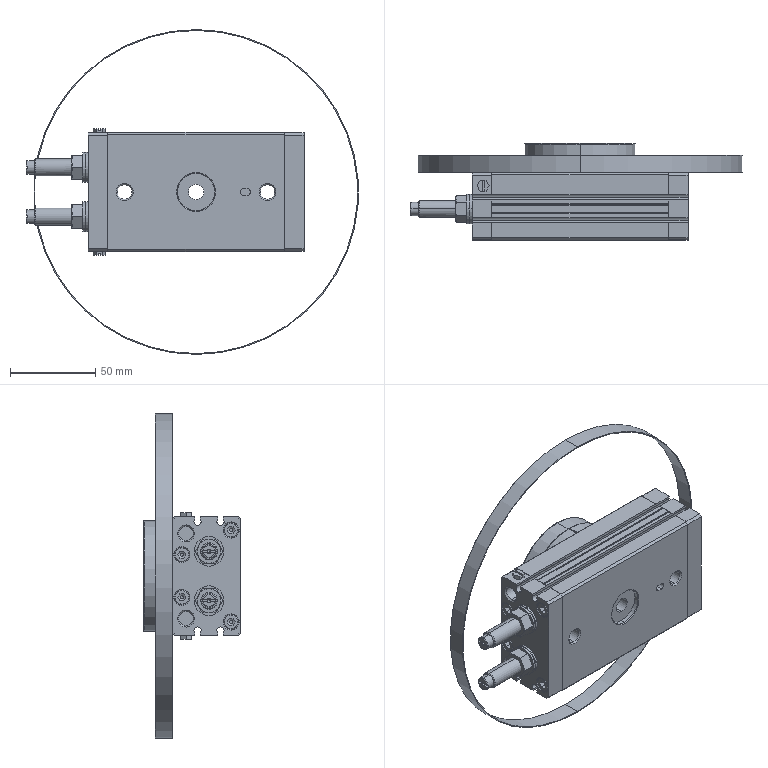Part | STEP file | 11-F12906-LQ-XZQG1A11 | 2 solids | 641 faces | box 195.5 x 57 x 191 mm | volume 392334 mm3 | plane 311 | cone 153 | cylinder 153 | spline 24 | commonest cylinder face diameters 4.917 x24 9 x18 8.5 x16 7.78 x12 8.28 x12 4 x8